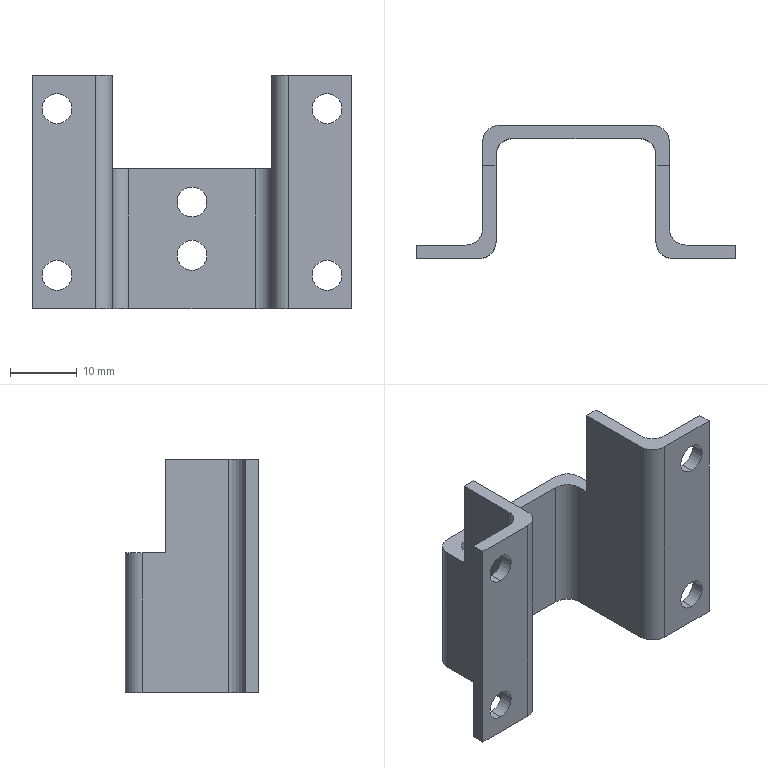Part | SolidWorks | features ICE 2, Extrusion 1 | 1 solid | 38 faces | box 48 x 20 x 35 mm | volume 4681 mm3 | cylinder 20 | plane 18 | commonest cylinder face diameters 4.5 x12 5 x8
STEP:
#1=CARTESIAN_POINT('',(0.,20.,5.75));
#2=VERTEX_POINT('',#1);
#3=CARTESIAN_POINT('',(0.,20.,10.25));
#4=VERTEX_POINT('',#3);
#5=CARTESIAN_POINT('',(0.,20.,8.));
#6=DIRECTION('',(0.,1.,0.));
#7=DIRECTION('',(0.,0.,-1.));
#8=AXIS2_PLACEMENT_3D('',#5,#6,#7);
#9=CIRCLE('',#8,2.25);
#10=EDGE_CURVE('',#2,#4,#9,.T.);
#11=ORIENTED_EDGE('',*,*,#10,.T.);
#12=CARTESIAN_POINT('',(0.,18.,10.25));
#13=VERTEX_POINT('',#12);
#14=CARTESIAN_POINT('',(0.,21.,10.25));
#15=DIRECTION('',(0.,-1.,0.));
#16=VECTOR('',#15,1000.);
#17=LINE('',#14,#16);
#18=EDGE_CURVE('',#4,#13,#17,.T.);
#19=ORIENTED_EDGE('',*,*,#18,.T.);
#20=CARTESIAN_POINT('',(0.,18.,5.75));
#21=VERTEX_POINT('',#20);
#22=CARTESIAN_POINT('',(0.,18.,8.));
#23=DIRECTION('',(0.,-1.,0.));
#24=DIRECTION('',(-1.,0.,0.));
#25=AXIS2_PLACEMENT_3D('',#22,#23,#24);
#26=CIRCLE('',#25,2.25);
#27=EDGE_CURVE('',#13,#21,#26,.T.);
#28=ORIENTED_EDGE('',*,*,#27,.T.);
#29=CARTESIAN_POINT('',(0.,21.,5.75));
#30=DIRECTION('',(0.,-1.,0.));
#31=VECTOR('',#30,1000.);
#32=LINE('',#29,#31);
#33=EDGE_CURVE('',#2,#21,#32,.T.);
#34=ORIENTED_EDGE('',*,*,#33,.F.);
#35=EDGE_LOOP('',(#11,#19,#28,#34));
#36=FACE_OUTER_BOUND('',#35,.T.);
#37=CARTESIAN_POINT('',(0.,21.,8.));
#38=DIRECTION('',(0.,-1.,0.));
#39=DIRECTION('',(0.,0.,-1.));
#40=AXIS2_PLACEMENT_3D('',#37,#38,#39);
#41=CYLINDRICAL_SURFACE('',#40,2.25);
#42=ADVANCED_FACE('',(#36),#41,.F.);
#43=CARTESIAN_POINT('',(0.,20.,13.75));
#44=VERTEX_POINT('',#43);
#45=CARTESIAN_POINT('',(0.,20.,18.25));
#46=VERTEX_POINT('',#45);
#47=CARTESIAN_POINT('',(0.,20.,16.));
#48=DIRECTION('',(0.,1.,0.));
#49=DIRECTION('',(0.,0.,-1.));
#50=AXIS2_PLACEMENT_3D('',#47,#48,#49);
#51=CIRCLE('',#50,2.25);
#52=EDGE_CURVE('',#44,#46,#51,.T.);
#53=ORIENTED_EDGE('',*,*,#52,.T.);
#54=CARTESIAN_POINT('',(0.,18.,18.25));
#55=VERTEX_POINT('',#54);
#56=CARTESIAN_POINT('',(0.,21.,18.25));
#57=DIRECTION('',(0.,-1.,0.));
#58=VECTOR('',#57,1000.);
#59=LINE('',#56,#58);
#60=EDGE_CURVE('',#46,#55,#59,.T.);
#61=ORIENTED_EDGE('',*,*,#60,.T.);
#62=CARTESIAN_POINT('',(0.,18.,13.75));
#63=VERTEX_POINT('',#62);
#64=CARTESIAN_POINT('',(0.,18.,16.));
#65=DIRECTION('',(0.,-1.,0.));
#66=DIRECTION('',(-1.,0.,0.));
#67=AXIS2_PLACEMENT_3D('',#64,#65,#66);
#68=CIRCLE('',#67,2.25);
#69=EDGE_CURVE('',#55,#63,#68,.T.);
#70=ORIENTED_EDGE('',*,*,#69,.T.);
#71=CARTESIAN_POINT('',(0.,21.,13.75));
#72=DIRECTION('',(0.,-1.,0.));
#73=VECTOR('',#72,1000.);
#74=LINE('',#71,#73);
#75=EDGE_CURVE('',#44,#63,#74,.T.);
#76=ORIENTED_EDGE('',*,*,#75,.F.);
#77=EDGE_LOOP('',(#53,#61,#70,#76));
#78=FACE_OUTER_BOUND('',#77,.T.);
#79=CARTESIAN_POINT('',(0.,21.,16.));
#80=DIRECTION('',(0.,-1.,0.));
#81=DIRECTION('',(0.,0.,-1.));
#82=AXIS2_PLACEMENT_3D('',#79,#80,#81);
#83=CYLINDRICAL_SURFACE('',#82,2.25);
#84=ADVANCED_FACE('',(#78),#83,.F.);
#85=CARTESIAN_POINT('',(20.25,2.,27.75));
#86=VERTEX_POINT('',#85);
#87=CARTESIAN_POINT('',(20.25,2.,32.25));
#88=VERTEX_POINT('',#87);
#89=CARTESIAN_POINT('',(20.25,2.,30.));
#90=DIRECTION('',(0.,1.,0.));
#91=DIRECTION('',(0.,0.,-1.));
#92=AXIS2_PLACEMENT_3D('',#89,#90,#91);
#93=CIRCLE('',#92,2.25);
#94=EDGE_CURVE('',#86,#88,#93,.T.);
#95=ORIENTED_EDGE('',*,*,#94,.T.);
#96=CARTESIAN_POINT('',(20.25,0.,32.25));
#97=VERTEX_POINT('',#96);
#98=CARTESIAN_POINT('',(20.25,21.,32.25));
#99=DIRECTION('',(0.,-1.,0.));
#100=VECTOR('',#99,1000.);
#101=LINE('',#98,#100);
#102=EDGE_CURVE('',#88,#97,#101,.T.);
#103=ORIENTED_EDGE('',*,*,#102,.T.);
#104=CARTESIAN_POINT('',(20.25,0.,27.75));
#105=VERTEX_POINT('',#104);
#106=CARTESIAN_POINT('',(20.25,0.,30.));
#107=DIRECTION('',(0.,-1.,0.));
#108=DIRECTION('',(-1.,0.,0.));
#109=AXIS2_PLACEMENT_3D('',#106,#107,#108);
#110=CIRCLE('',#109,2.25);
#111=EDGE_CURVE('',#97,#105,#110,.T.);
#112=ORIENTED_EDGE('',*,*,#111,.T.);
#113=CARTESIAN_POINT('',(20.25,21.,27.75));
#114=DIRECTION('',(0.,-1.,0.));
#115=VECTOR('',#114,1000.);
#116=LINE('',#113,#115);
#117=EDGE_CURVE('',#86,#105,#116,.T.);
#118=ORIENTED_EDGE('',*,*,#117,.F.);
#119=EDGE_LOOP('',(#95,#103,#112,#118));
#120=FACE_OUTER_BOUND('',#119,.T.);
#121=CARTESIAN_POINT('',(20.25,21.,30.));
#122=DIRECTION('',(0.,-1.,0.));
#123=DIRECTION('',(0.,0.,-1.));
#124=AXIS2_PLACEMENT_3D('',#121,#122,#123);
#125=CYLINDRICAL_SURFACE('',#124,2.25);
#126=ADVANCED_FACE('',(#120),#125,.F.);
#127=CARTESIAN_POINT('',(20.25,2.,2.75));
#128=VERTEX_POINT('',#127);
#129=CARTESIAN_POINT('',(20.25,2.,7.25));
#130=VERTEX_POINT('',#129);
#131=CARTESIAN_POINT('',(20.25,2.,5.));
#132=DIRECTION('',(0.,1.,0.));
#133=DIRECTION('',(0.,0.,-1.));
#134=AXIS2_PLACEMENT_3D('',#131,#132,#133);
#135=CIRCLE('',#134,2.25);
#136=EDGE_CURVE('',#128,#130,#135,.T.);
#137=ORIENTED_EDGE('',*,*,#136,.T.);
#138=CARTESIAN_POINT('',(20.25,0.,7.25));
#139=VERTEX_POINT('',#138);
#140=CARTESIAN_POINT('',(20.25,21.,7.25));
#141=DIRECTION('',(0.,-1.,0.));
#142=VECTOR('',#141,1000.);
#143=LINE('',#140,#142);
#144=EDGE_CURVE('',#130,#139,#143,.T.);
#145=ORIENTED_EDGE('',*,*,#144,.T.);
#146=CARTESIAN_POINT('',(20.25,0.,2.75));
#147=VERTEX_POINT('',#146);
#148=CARTESIAN_POINT('',(20.25,0.,5.));
#149=DIRECTION('',(0.,-1.,0.));
#150=DIRECTION('',(-1.,0.,0.));
#151=AXIS2_PLACEMENT_3D('',#148,#149,#150);
#152=CIRCLE('',#151,2.25);
#153=EDGE_CURVE('',#139,#147,#152,.T.);
#154=ORIENTED_EDGE('',*,*,#153,.T.);
#155=CARTESIAN_POINT('',(20.25,21.,2.75));
#156=DIRECTION('',(0.,-1.,0.));
#157=VECTOR('',#156,1000.);
#158=LINE('',#155,#157);
#159=EDGE_CURVE('',#128,#147,#158,.T.);
#160=ORIENTED_EDGE('',*,*,#159,.F.);
#161=EDGE_LOOP('',(#137,#145,#154,#160));
#162=FACE_OUTER_BOUND('',#161,.T.);
#163=CARTESIAN_POINT('',(20.25,21.,5.));
#164=DIRECTION('',(0.,-1.,0.));
#165=DIRECTION('',(0.,0.,-1.));
#166=AXIS2_PLACEMENT_3D('',#163,#164,#165);
#167=CYLINDRICAL_SURFACE('',#166,2.25);
#168=ADVANCED_FACE('',(#162),#167,.F.);
#169=CARTESIAN_POINT('',(-20.25,2.,27.75));
#170=VERTEX_POINT('',#169);
#171=CARTESIAN_POINT('',(-20.25,2.,32.25));
#172=VERTEX_POINT('',#171);
#173=CARTESIAN_POINT('',(-20.25,2.,30.));
#174=DIRECTION('',(0.,1.,0.));
#175=DIRECTION('',(0.,0.,-1.));
#176=AXIS2_PLACEMENT_3D('',#173,#174,#175);
#177=CIRCLE('',#176,2.25);
#178=EDGE_CURVE('',#170,#172,#177,.T.);
#179=ORIENTED_EDGE('',*,*,#178,.T.);
#180=CARTESIAN_POINT('',(-20.25,0.,32.25));
#181=VERTEX_POINT('',#180);
#182=CARTESIAN_POINT('',(-20.25,21.,32.25));
#183=DIRECTION('',(0.,-1.,0.));
#184=VECTOR('',#183,1000.);
#185=LINE('',#182,#184);
#186=EDGE_CURVE('',#172,#181,#185,.T.);
#187=ORIENTED_EDGE('',*,*,#186,.T.);
#188=CARTESIAN_POINT('',(-20.25,0.,27.75));
#189=VERTEX_POINT('',#188);
#190=CARTESIAN_POINT('',(-20.25,0.,30.));
#191=DIRECTION('',(0.,-1.,0.));
#192=DIRECTION('',(0.,0.,1.));
#193=AXIS2_PLACEMENT_3D('',#190,#191,#192);
#194=CIRCLE('',#193,2.25);
#195=EDGE_CURVE('',#181,#189,#194,.T.);
#196=ORIENTED_EDGE('',*,*,#195,.T.);
#197=CARTESIAN_POINT('',(-20.25,21.,27.75));
#198=DIRECTION('',(0.,-1.,0.));
#199=VECTOR('',#198,1000.);
#200=LINE('',#197,#199);
#201=EDGE_CURVE('',#170,#189,#200,.T.);
#202=ORIENTED_EDGE('',*,*,#201,.F.);
#203=EDGE_LOOP('',(#179,#187,#196,#202));
#204=FACE_OUTER_BOUND('',#203,.T.);
#205=CARTESIAN_POINT('',(-20.25,21.,30.));
#206=DIRECTION('',(0.,-1.,0.));
#207=DIRECTION('',(0.,0.,-1.));
#208=AXIS2_PLACEMENT_3D('',#205,#206,#207);
#209=CYLINDRICAL_SURFACE('',#208,2.25);
#210=ADVANCED_FACE('',(#204),#209,.F.);
#211=CARTESIAN_POINT('',(-20.25,2.,2.75));
#212=VERTEX_POINT('',#211);
#213=CARTESIAN_POINT('',(-20.25,2.,7.25));
#214=VERTEX_POINT('',#213);
#215=CARTESIAN_POINT('',(-20.25,2.,5.));
#216=DIRECTION('',(0.,1.,0.));
#217=DIRECTION('',(0.,0.,-1.));
#218=AXIS2_PLACEMENT_3D('',#215,#216,#217);
#219=CIRCLE('',#218,2.25);
#220=EDGE_CURVE('',#212,#214,#219,.T.);
#221=ORIENTED_EDGE('',*,*,#220,.T.);
#222=CARTESIAN_POINT('',(-20.25,0.,7.25));
#223=VERTEX_POINT('',#222);
#224=CARTESIAN_POINT('',(-20.25,21.,7.25));
#225=DIRECTION('',(0.,-1.,0.));
#226=VECTOR('',#225,1000.);
#227=LINE('',#224,#226);
#228=EDGE_CURVE('',#214,#223,#227,.T.);
#229=ORIENTED_EDGE('',*,*,#228,.T.);
#230=CARTESIAN_POINT('',(-20.25,0.,2.75));
#231=VERTEX_POINT('',#230);
#232=CARTESIAN_POINT('',(-20.25,0.,5.));
#233=DIRECTION('',(0.,-1.,0.));
#234=DIRECTION('',(0.,0.,1.));
#235=AXIS2_PLACEMENT_3D('',#232,#233,#234);
#236=CIRCLE('',#235,2.25);
#237=EDGE_CURVE('',#223,#231,#236,.T.);
#238=ORIENTED_EDGE('',*,*,#237,.T.);
#239=CARTESIAN_POINT('',(-20.25,21.,2.75));
#240=DIRECTION('',(0.,-1.,0.));
#241=VECTOR('',#240,1000.);
#242=LINE('',#239,#241);
#243=EDGE_CURVE('',#212,#231,#242,.T.);
#244=ORIENTED_EDGE('',*,*,#243,.F.);
#245=EDGE_LOOP('',(#221,#229,#238,#244));
#246=FACE_OUTER_BOUND('',#245,.T.);
#247=CARTESIAN_POINT('',(-20.25,21.,5.));
#248=DIRECTION('',(0.,-1.,0.));
#249=DIRECTION('',(0.,0.,-1.));
#250=AXIS2_PLACEMENT_3D('',#247,#248,#249);
#251=CYLINDRICAL_SURFACE('',#250,2.25);
#252=ADVANCED_FACE('',(#246),#251,.F.);
#253=CARTESIAN_POINT('',(-12.,15.5,21.));
#254=VERTEX_POINT('',#253);
#255=CARTESIAN_POINT('',(-9.5,18.,21.));
#256=VERTEX_POINT('',#255);
#257=CARTESIAN_POINT('',(-9.5,15.5,21.));
#258=DIRECTION('',(0.,0.,-1.));
#259=DIRECTION('',(1.,0.,0.));
#260=AXIS2_PLACEMENT_3D('',#257,#258,#259);
#261=CIRCLE('',#260,2.5);
#262=EDGE_CURVE('',#254,#256,#261,.T.);
#263=ORIENTED_EDGE('',*,*,#262,.F.);
#264=CARTESIAN_POINT('',(-12.,15.5,0.));
#265=VERTEX_POINT('',#264);
#266=CARTESIAN_POINT('',(-12.,15.5,35.));
#267=DIRECTION('',(0.,0.,-1.));
#268=VECTOR('',#267,1000.);
#269=LINE('',#266,#268);
#270=EDGE_CURVE('',#254,#265,#269,.T.);
#271=ORIENTED_EDGE('',*,*,#270,.T.);
#272=CARTESIAN_POINT('',(-9.5,18.,0.));
#273=VERTEX_POINT('',#272);
#274=CARTESIAN_POINT('',(-9.5,15.5,0.));
#275=DIRECTION('',(0.,0.,-1.));
#276=DIRECTION('',(-1.,0.,0.));
#277=AXIS2_PLACEMENT_3D('',#274,#275,#276);
#278=CIRCLE('',#277,2.5);
#279=EDGE_CURVE('',#265,#273,#278,.T.);
#280=ORIENTED_EDGE('',*,*,#279,.T.);
#281=CARTESIAN_POINT('',(-9.5,18.,35.));
#282=DIRECTION('',(0.,0.,-1.));
#283=VECTOR('',#282,1000.);
#284=LINE('',#281,#283);
#285=EDGE_CURVE('',#256,#273,#284,.T.);
#286=ORIENTED_EDGE('',*,*,#285,.F.);
#287=EDGE_LOOP('',(#263,#271,#280,#286));
#288=FACE_OUTER_BOUND('',#287,.T.);
#289=CARTESIAN_POINT('',(-9.5,15.5,35.));
#290=DIRECTION('',(0.,0.,-1.));
#291=DIRECTION('',(-1.,0.,0.));
#292=AXIS2_PLACEMENT_3D('',#289,#290,#291);
#293=CYLINDRICAL_SURFACE('',#292,2.5);
#294=ADVANCED_FACE('',(#288),#293,.F.);
#295=CARTESIAN_POINT('',(0.,18.,8.));
#296=DIRECTION('',(0.,-1.,0.));
#297=DIRECTION('',(-1.,0.,0.));
#298=AXIS2_PLACEMENT_3D('',#295,#296,#297);
#299=CIRCLE('',#298,2.25);
#300=EDGE_CURVE('',#21,#13,#299,.T.);
#301=ORIENTED_EDGE('',*,*,#300,.F.);
#302=ORIENTED_EDGE('',*,*,#27,.F.);
#303=EDGE_LOOP('',(#301,#302));
#304=FACE_BOUND('',#303,.T.);
#305=CARTESIAN_POINT('',(0.,18.,16.));
#306=DIRECTION('',(0.,-1.,0.));
#307=DIRECTION('',(-1.,0.,0.));
#308=AXIS2_PLACEMENT_3D('',#305,#306,#307);
#309=CIRCLE('',#308,2.25);
#310=EDGE_CURVE('',#63,#55,#309,.T.);
#311=ORIENTED_EDGE('',*,*,#310,.F.);
#312=ORIENTED_EDGE('',*,*,#69,.F.);
#313=EDGE_LOOP('',(#311,#312));
#314=FACE_BOUND('',#313,.T.);
#315=CARTESIAN_POINT('',(9.5,18.,21.));
#316=VERTEX_POINT('',#315);
#317=CARTESIAN_POINT('',(-9.5,18.,21.));
#318=DIRECTION('',(1.,0.,0.));
#319=VECTOR('',#318,1000.);
#320=LINE('',#317,#319);
#321=EDGE_CURVE('',#256,#316,#320,.T.);
#322=ORIENTED_EDGE('',*,*,#321,.F.);
#323=ORIENTED_EDGE('',*,*,#285,.T.);
#324=CARTESIAN_POINT('',(9.5,18.,0.));
#325=VERTEX_POINT('',#324);
#326=CARTESIAN_POINT('',(-9.5,18.,0.));
#327=DIRECTION('',(1.,0.,0.));
#328=VECTOR('',#327,1000.);
#329=LINE('',#326,#328);
#330=EDGE_CURVE('',#273,#325,#329,.T.);
#331=ORIENTED_EDGE('',*,*,#330,.T.);
#332=CARTESIAN_POINT('',(9.5,18.,35.));
#333=DIRECTION('',(0.,0.,-1.));
#334=VECTOR('',#333,1000.);
#335=LINE('',#332,#334);
#336=EDGE_CURVE('',#316,#325,#335,.T.);
#337=ORIENTED_EDGE('',*,*,#336,.F.);
#338=EDGE_LOOP('',(#322,#323,#331,#337));
#339=FACE_OUTER_BOUND('',#338,.T.);
#340=CARTESIAN_POINT('',(-9.5,18.,35.));
#341=DIRECTION('',(0.,1.,0.));
#342=DIRECTION('',(-1.,0.,0.));
#343=AXIS2_PLACEMENT_3D('',#340,#341,#342);
#344=PLANE('',#343);
#345=ADVANCED_FACE('',(#304,#314,#339),#344,.F.);
#346=CARTESIAN_POINT('',(12.,15.5,21.));
#347=VERTEX_POINT('',#346);
#348=CARTESIAN_POINT('',(9.5,15.5,21.));
#349=DIRECTION('',(0.,0.,-1.));
#350=DIRECTION('',(1.,0.,0.));
#351=AXIS2_PLACEMENT_3D('',#348,#349,#350);
#352=CIRCLE('',#351,2.5);
#353=EDGE_CURVE('',#316,#347,#352,.T.);
#354=ORIENTED_EDGE('',*,*,#353,.F.);
#355=ORIENTED_EDGE('',*,*,#336,.T.);
#356=CARTESIAN_POINT('',(12.,15.5,0.));
#357=VERTEX_POINT('',#356);
#358=CARTESIAN_POINT('',(9.5,15.5,0.));
#359=DIRECTION('',(0.,0.,-1.));
#360=DIRECTION('',(1.,0.,0.));
#361=AXIS2_PLACEMENT_3D('',#358,#359,#360);
#362=CIRCLE('',#361,2.5);
#363=EDGE_CURVE('',#325,#357,#362,.T.);
#364=ORIENTED_EDGE('',*,*,#363,.T.);
#365=CARTESIAN_POINT('',(12.,15.5,35.));
#366=DIRECTION('',(0.,0.,-1.));
#367=VECTOR('',#366,1000.);
#368=LINE('',#365,#367);
#369=EDGE_CURVE('',#347,#357,#368,.T.);
#370=ORIENTED_EDGE('',*,*,#369,.F.);
#371=EDGE_LOOP('',(#354,#355,#364,#370));
#372=FACE_OUTER_BOUND('',#371,.T.);
#373=CARTESIAN_POINT('',(9.5,15.5,35.));
#374=DIRECTION('',(0.,0.,-1.));
#375=DIRECTION('',(-1.,0.,0.));
#376=AXIS2_PLACEMENT_3D('',#373,#374,#375);
#377=CYLINDRICAL_SURFACE('',#376,2.5);
#378=ADVANCED_FACE('',(#372),#377,.F.);
#379=CARTESIAN_POINT('',(14.,17.5,21.));
#380=VERTEX_POINT('',#379);
#381=CARTESIAN_POINT('',(11.5,20.,21.));
#382=VERTEX_POINT('',#381);
#383=CARTESIAN_POINT('',(11.5,17.5,21.));
#384=DIRECTION('',(0.,0.,1.));
#385=DIRECTION('',(1.,0.,0.));
#386=AXIS2_PLACEMENT_3D('',#383,#384,#385);
#387=CIRCLE('',#386,2.5);
#388=EDGE_CURVE('',#380,#382,#387,.T.);
#389=ORIENTED_EDGE('',*,*,#388,.F.);
#390=CARTESIAN_POINT('',(14.,17.5,0.));
#391=VERTEX_POINT('',#390);
#392=CARTESIAN_POINT('',(14.,17.5,35.));
#393=DIRECTION('',(0.,0.,-1.));
#394=VECTOR('',#393,1000.);
#395=LINE('',#392,#394);
#396=EDGE_CURVE('',#380,#391,#395,.T.);
#397=ORIENTED_EDGE('',*,*,#396,.T.);
#398=CARTESIAN_POINT('',(11.5,20.,0.));
#399=VERTEX_POINT('',#398);
#400=CARTESIAN_POINT('',(11.5,17.5,0.));
#401=DIRECTION('',(0.,0.,1.));
#402=DIRECTION('',(1.,0.,0.));
#403=AXIS2_PLACEMENT_3D('',#400,#401,#402);
#404=CIRCLE('',#403,2.5);
#405=EDGE_CURVE('',#391,#399,#404,.T.);
#406=ORIENTED_EDGE('',*,*,#405,.T.);
#407=CARTESIAN_POINT('',(11.5,20.,35.));
#408=DIRECTION('',(0.,0.,-1.));
#409=VECTOR('',#408,1000.);
#410=LINE('',#407,#409);
#411=EDGE_CURVE('',#382,#399,#410,.T.);
#412=ORIENTED_EDGE('',*,*,#411,.F.);
#413=EDGE_LOOP('',(#389,#397,#406,#412));
#414=FACE_OUTER_BOUND('',#413,.T.);
#415=CARTESIAN_POINT('',(11.5,17.5,35.));
#416=DIRECTION('',(0.,0.,-1.));
#417=DIRECTION('',(-1.,0.,0.));
#418=AXIS2_PLACEMENT_3D('',#415,#416,#417);
#419=CYLINDRICAL_SURFACE('',#418,2.5);
#420=ADVANCED_FACE('',(#414),#419,.T.);
#421=ORIENTED_EDGE('',*,*,#10,.F.);
#422=CARTESIAN_POINT('',(0.,20.,8.));
#423=DIRECTION('',(0.,1.,0.));
#424=DIRECTION('',(0.,0.,-1.));
#425=AXIS2_PLACEMENT_3D('',#422,#423,#424);
#426=CIRCLE('',#425,2.25);
#427=EDGE_CURVE('',#4,#2,#426,.T.);
#428=ORIENTED_EDGE('',*,*,#427,.F.);
#429=EDGE_LOOP('',(#421,#428));
#430=FACE_BOUND('',#429,.T.);
#431=ORIENTED_EDGE('',*,*,#52,.F.);
#432=CARTESIAN_POINT('',(0.,20.,16.));
#433=DIRECTION('',(0.,1.,0.));
#434=DIRECTION('',(0.,0.,-1.));
#435=AXIS2_PLACEMENT_3D('',#432,#433,#434);
#436=CIRCLE('',#435,2.25);
#437=EDGE_CURVE('',#46,#44,#436,.T.);
#438=ORIENTED_EDGE('',*,*,#437,.F.);
#439=EDGE_LOOP('',(#431,#438));
#440=FACE_BOUND('',#439,.T.);
#441=CARTESIAN_POINT('',(-11.5,20.,21.));
#442=VERTEX_POINT('',#441);
#443=CARTESIAN_POINT('',(-11.5,20.,21.));
#444=DIRECTION('',(-1.,0.,0.));
#445=VECTOR('',#444,1000.);
#446=LINE('',#443,#445);
#447=EDGE_CURVE('',#382,#442,#446,.T.);
#448=ORIENTED_EDGE('',*,*,#447,.F.);
#449=ORIENTED_EDGE('',*,*,#411,.T.);
#450=CARTESIAN_POINT('',(-11.5,20.,0.));
#451=VERTEX_POINT('',#450);
#452=CARTESIAN_POINT('',(-11.5,20.,0.));
#453=DIRECTION('',(-1.,0.,0.));
#454=VECTOR('',#453,1000.);
#455=LINE('',#452,#454);
#456=EDGE_CURVE('',#399,#451,#455,.T.);
#457=ORIENTED_EDGE('',*,*,#456,.T.);
#458=CARTESIAN_POINT('',(-11.5,20.,35.));
#459=DIRECTION('',(0.,0.,-1.));
#460=VECTOR('',#459,1000.);
#461=LINE('',#458,#460);
#462=EDGE_CURVE('',#442,#451,#461,.T.);
#463=ORIENTED_EDGE('',*,*,#462,.F.);
#464=EDGE_LOOP('',(#448,#449,#457,#463));
#465=FACE_OUTER_BOUND('',#464,.T.);
#466=CARTESIAN_POINT('',(-11.5,20.,35.));
#467=DIRECTION('',(0.,-1.,0.));
#468=DIRECTION('',(0.,0.,-1.));
#469=AXIS2_PLACEMENT_3D('',#466,#467,#468);
#470=PLANE('',#469);
#471=ADVANCED_FACE('',(#430,#440,#465),#470,.F.);
#472=CARTESIAN_POINT('',(-14.,17.5,21.));
#473=VERTEX_POINT('',#472);
#474=CARTESIAN_POINT('',(-11.5,17.5,21.));
#475=DIRECTION('',(0.,0.,1.));
#476=DIRECTION('',(1.,0.,0.));
#477=AXIS2_PLACEMENT_3D('',#474,#475,#476);
#478=CIRCLE('',#477,2.5);
#479=EDGE_CURVE('',#442,#473,#478,.T.);
#480=ORIENTED_EDGE('',*,*,#479,.F.);
#481=ORIENTED_EDGE('',*,*,#462,.T.);
#482=CARTESIAN_POINT('',(-14.,17.5,0.));
#483=VERTEX_POINT('',#482);
#484=CARTESIAN_POINT('',(-11.5,17.5,0.));
#485=DIRECTION('',(0.,0.,1.));
#486=DIRECTION('',(-1.,0.,0.));
#487=AXIS2_PLACEMENT_3D('',#484,#485,#486);
#488=CIRCLE('',#487,2.5);
#489=EDGE_CURVE('',#451,#483,#488,.T.);
#490=ORIENTED_EDGE('',*,*,#489,.T.);
#491=CARTESIAN_POINT('',(-14.,17.5,35.));
#492=DIRECTION('',(0.,0.,-1.));
#493=VECTOR('',#492,1000.);
#494=LINE('',#491,#493);
#495=EDGE_CURVE('',#473,#483,#494,.T.);
#496=ORIENTED_EDGE('',*,*,#495,.F.);
#497=EDGE_LOOP('',(#480,#481,#490,#496));
#498=FACE_OUTER_BOUND('',#497,.T.);
#499=CARTESIAN_POINT('',(-11.5,17.5,35.));
#500=DIRECTION('',(0.,0.,-1.));
#501=DIRECTION('',(-1.,0.,0.));
#502=AXIS2_PLACEMENT_3D('',#499,#500,#501);
#503=CYLINDRICAL_SURFACE('',#502,2.5);
#504=ADVANCED_FACE('',(#498),#503,.T.);
#505=CARTESIAN_POINT('',(-14.,14.,35.));
#506=VERTEX_POINT('',#505);
#507=CARTESIAN_POINT('',(-12.,14.,35.));
#508=VERTEX_POINT('',#507);
#509=CARTESIAN_POINT('',(-14.5,14.,35.));
#510=DIRECTION('',(1.,0.,0.));
#511=VECTOR('',#510,1000.);
#512=LINE('',#509,#511);
#513=EDGE_CURVE('',#506,#508,#512,.T.);
#514=ORIENTED_EDGE('',*,*,#513,.F.);
#515=CARTESIAN_POINT('',(-14.,4.5,35.));
#516=VERTEX_POINT('',#515);
#517=CARTESIAN_POINT('',(-14.,4.5,35.));
#518=DIRECTION('',(0.,-1.,0.));
#519=VECTOR('',#518,1000.);
#520=LINE('',#517,#519);
#521=EDGE_CURVE('',#506,#516,#520,.T.);
#522=ORIENTED_EDGE('',*,*,#521,.T.);
#523=CARTESIAN_POINT('',(-16.5,2.,35.));
#524=VERTEX_POINT('',#523);
#525=CARTESIAN_POINT('',(-16.5,4.5,35.));
#526=DIRECTION('',(0.,0.,-1.));
#527=DIRECTION('',(1.,0.,0.));
#528=AXIS2_PLACEMENT_3D('',#525,#526,#527);
#529=CIRCLE('',#528,2.5);
#530=EDGE_CURVE('',#516,#524,#529,.T.);
#531=ORIENTED_EDGE('',*,*,#530,.T.);
#532=CARTESIAN_POINT('',(-24.,2.,35.));
#533=VERTEX_POINT('',#532);
#534=CARTESIAN_POINT('',(-24.,2.,35.));
#535=DIRECTION('',(-1.,0.,0.));
#536=VECTOR('',#535,1000.);
#537=LINE('',#534,#536);
#538=EDGE_CURVE('',#524,#533,#537,.T.);
#539=ORIENTED_EDGE('',*,*,#538,.T.);
#540=CARTESIAN_POINT('',(-24.,0.,35.));
#541=VERTEX_POINT('',#540);
#542=CARTESIAN_POINT('',(-24.,2.,35.));
#543=DIRECTION('',(0.,-1.,0.));
#544=VECTOR('',#543,1000.);
#545=LINE('',#542,#544);
#546=EDGE_CURVE('',#533,#541,#545,.T.);
#547=ORIENTED_EDGE('',*,*,#546,.T.);
#548=CARTESIAN_POINT('',(-14.5,0.,35.));
#549=VERTEX_POINT('',#548);
#550=CARTESIAN_POINT('',(-24.,0.,35.));
#551=DIRECTION('',(1.,0.,0.));
#552=VECTOR('',#551,1000.);
#553=LINE('',#550,#552);
#554=EDGE_CURVE('',#541,#549,#553,.T.);
#555=ORIENTED_EDGE('',*,*,#554,.T.);
#556=CARTESIAN_POINT('',(-12.,2.5,35.));
#557=VERTEX_POINT('',#556);
#558=CARTESIAN_POINT('',(-14.5,2.5,35.));
#559=DIRECTION('',(0.,0.,1.));
#560=DIRECTION('',(1.,0.,0.));
#561=AXIS2_PLACEMENT_3D('',#558,#559,#560);
#562=CIRCLE('',#561,2.5);
#563=EDGE_CURVE('',#549,#557,#562,.T.);
#564=ORIENTED_EDGE('',*,*,#563,.T.);
#565=CARTESIAN_POINT('',(-12.,2.5,35.));
#566=DIRECTION('',(0.,1.,0.));
#567=VECTOR('',#566,1000.);
#568=LINE('',#565,#567);
#569=EDGE_CURVE('',#557,#508,#568,.T.);
#570=ORIENTED_EDGE('',*,*,#569,.T.);
#571=EDGE_LOOP('',(#514,#522,#531,#539,#547,#555,#564,#570));
#572=FACE_OUTER_BOUND('',#571,.T.);
#573=CARTESIAN_POINT('',(-14.5,2.5,35.));
#574=DIRECTION('',(0.,0.,1.));
#575=DIRECTION('',(1.,0.,0.));
#576=AXIS2_PLACEMENT_3D('',#573,#574,#575);
#577=PLANE('',#576);
#578=ADVANCED_FACE('',(#572),#577,.T.);
#579=CARTESIAN_POINT('',(-24.,2.,0.));
#580=VERTEX_POINT('',#579);
#581=CARTESIAN_POINT('',(-24.,0.,0.));
#582=VERTEX_POINT('',#581);
#583=CARTESIAN_POINT('',(-24.,2.,0.));
#584=DIRECTION('',(0.,-1.,0.));
#585=VECTOR('',#584,1000.);
#586=LINE('',#583,#585);
#587=EDGE_CURVE('',#580,#582,#586,.T.);
#588=ORIENTED_EDGE('',*,*,#587,.T.);
#589=CARTESIAN_POINT('',(-24.,0.,35.));
#590=DIRECTION('',(0.,0.,-1.));
#591=VECTOR('',#590,1000.);
#592=LINE('',#589,#591);
#593=EDGE_CURVE('',#541,#582,#592,.T.);
#594=ORIENTED_EDGE('',*,*,#593,.F.);
#595=ORIENTED_EDGE('',*,*,#546,.F.);
#596=CARTESIAN_POINT('',(-24.,2.,35.));
#597=DIRECTION('',(0.,0.,-1.));
#598=VECTOR('',#597,1000.);
#599=LINE('',#596,#598);
#600=EDGE_CURVE('',#533,#580,#599,.T.);
#601=ORIENTED_EDGE('',*,*,#600,.T.);
#602=EDGE_LOOP('',(#588,#594,#595,#601));
#603=FACE_OUTER_BOUND('',#602,.T.);
#604=CARTESIAN_POINT('',(-24.,2.,35.));
#605=DIRECTION('',(1.,0.,0.));
#606=DIRECTION('',(0.,0.,-1.));
#607=AXIS2_PLACEMENT_3D('',#604,#605,#606);
#608=PLANE('',#607);
#609=ADVANCED_FACE('',(#603),#608,.F.);
#610=CARTESIAN_POINT('',(-20.25,0.,30.));
#611=DIRECTION('',(0.,-1.,0.));
#612=DIRECTION('',(0.,0.,1.));
#613=AXIS2_PLACEMENT_3D('',#610,#611,#612);
#614=CIRCLE('',#613,2.25);
#615=EDGE_CURVE('',#189,#181,#614,.T.);
#616=ORIENTED_EDGE('',*,*,#615,.F.);
#617=ORIENTED_EDGE('',*,*,#195,.F.);
#618=EDGE_LOOP('',(#616,#617));
#619=FACE_BOUND('',#618,.T.);
#620=CARTESIAN_POINT('',(-20.25,0.,5.));
#621=DIRECTION('',(0.,-1.,0.));
#622=DIRECTION('',(0.,0.,1.));
#623=AXIS2_PLACEMENT_3D('',#620,#621,#622);
#624=CIRCLE('',#623,2.25);
#625=EDGE_CURVE('',#231,#223,#624,.T.);
#626=ORIENTED_EDGE('',*,*,#625,.F.);
#627=ORIENTED_EDGE('',*,*,#237,.F.);
#628=EDGE_LOOP('',(#626,#627));
#629=FACE_BOUND('',#628,.T.);
#630=CARTESIAN_POINT('',(-14.5,0.,0.));
#631=VERTEX_POINT('',#630);
#632=CARTESIAN_POINT('',(-24.,0.,0.));
#633=DIRECTION('',(1.,0.,0.));
#634=VECTOR('',#633,1000.);
#635=LINE('',#632,#634);
#636=EDGE_CURVE('',#582,#631,#635,.T.);
#637=ORIENTED_EDGE('',*,*,#636,.T.);
#638=CARTESIAN_POINT('',(-14.5,0.,35.));
#639=DIRECTION('',(0.,0.,-1.));
#640=VECTOR('',#639,1000.);
#641=LINE('',#638,#640);
#642=EDGE_CURVE('',#549,#631,#641,.T.);
#643=ORIENTED_EDGE('',*,*,#642,.F.);
#644=ORIENTED_EDGE('',*,*,#554,.F.);
#645=ORIENTED_EDGE('',*,*,#593,.T.);
#646=EDGE_LOOP('',(#637,#643,#644,#645));
#647=FACE_OUTER_BOUND('',#646,.T.);
#648=CARTESIAN_POINT('',(-24.,0.,35.));
#649=DIRECTION('',(0.,1.,0.));
#650=DIRECTION('',(0.,0.,1.));
#651=AXIS2_PLACEMENT_3D('',#648,#649,#650);
#652=PLANE('',#651);
#653=ADVANCED_FACE('',(#619,#629,#647),#652,.F.);
#654=CARTESIAN_POINT('',(-12.,2.5,0.));
#655=VERTEX_POINT('',#654);
#656=CARTESIAN_POINT('',(-14.5,2.5,0.));
#657=DIRECTION('',(0.,0.,1.));
#658=DIRECTION('',(1.,0.,0.));
#659=AXIS2_PLACEMENT_3D('',#656,#657,#658);
#660=CIRCLE('',#659,2.5);
#661=EDGE_CURVE('',#631,#655,#660,.T.);
#662=ORIENTED_EDGE('',*,*,#661,.T.);
#663=CARTESIAN_POINT('',(-12.,2.5,35.));
#664=DIRECTION('',(0.,0.,-1.));
#665=VECTOR('',#664,1000.);
#666=LINE('',#663,#665);
#667=EDGE_CURVE('',#557,#655,#666,.T.);
#668=ORIENTED_EDGE('',*,*,#667,.F.);
#669=ORIENTED_EDGE('',*,*,#563,.F.);
#670=ORIENTED_EDGE('',*,*,#642,.T.);
#671=EDGE_LOOP('',(#662,#668,#669,#670));
#672=FACE_OUTER_BOUND('',#671,.T.);
#673=CARTESIAN_POINT('',(-14.5,2.5,35.));
#674=DIRECTION('',(0.,0.,-1.));
#675=DIRECTION('',(-1.,0.,0.));
#676=AXIS2_PLACEMENT_3D('',#673,#674,#675);
#677=CYLINDRICAL_SURFACE('',#676,2.5);
#678=ADVANCED_FACE('',(#672),#677,.T.);
#679=CARTESIAN_POINT('',(-12.,14.,21.));
#680=VERTEX_POINT('',#679);
#681=CARTESIAN_POINT('',(-12.,2.5,21.));
#682=DIRECTION('',(0.,1.,0.));
#683=VECTOR('',#682,1000.);
#684=LINE('',#681,#683);
#685=EDGE_CURVE('',#680,#254,#684,.T.);
#686=ORIENTED_EDGE('',*,*,#685,.F.);
#687=CARTESIAN_POINT('',(-12.,14.,35.));
#688=DIRECTION('',(0.,0.,1.));
#689=VECTOR('',#688,1000.);
#690=LINE('',#687,#689);
#691=EDGE_CURVE('',#680,#508,#690,.T.);
#692=ORIENTED_EDGE('',*,*,#691,.T.);
#693=ORIENTED_EDGE('',*,*,#569,.F.);
#694=ORIENTED_EDGE('',*,*,#667,.T.);
#695=CARTESIAN_POINT('',(-12.,2.5,0.));
#696=DIRECTION('',(0.,1.,0.));
#697=VECTOR('',#696,1000.);
#698=LINE('',#695,#697);
#699=EDGE_CURVE('',#655,#265,#698,.T.);
#700=ORIENTED_EDGE('',*,*,#699,.T.);
#701=ORIENTED_EDGE('',*,*,#270,.F.);
#702=EDGE_LOOP('',(#686,#692,#693,#694,#700,#701));
#703=FACE_OUTER_BOUND('',#702,.T.);
#704=CARTESIAN_POINT('',(-12.,2.5,35.));
#705=DIRECTION('',(-1.,0.,0.));
#706=DIRECTION('',(0.,0.,1.));
#707=AXIS2_PLACEMENT_3D('',#704,#705,#706);
#708=PLANE('',#707);
#709=ADVANCED_FACE('',(#703),#708,.F.);
#710=CARTESIAN_POINT('',(12.,14.,35.));
#711=VERTEX_POINT('',#710);
#712=CARTESIAN_POINT('',(12.,2.5,35.));
#713=VERTEX_POINT('',#712);
#714=CARTESIAN_POINT('',(12.,15.5,35.));
#715=DIRECTION('',(0.,-1.,0.));
#716=VECTOR('',#715,1000.);
#717=LINE('',#714,#716);
#718=EDGE_CURVE('',#711,#713,#717,.T.);
#719=ORIENTED_EDGE('',*,*,#718,.F.);
#720=CARTESIAN_POINT('',(12.,14.,21.));
#721=VERTEX_POINT('',#720);
#722=CARTESIAN_POINT('',(12.,14.,35.));
#723=DIRECTION('',(0.,0.,-1.));
#724=VECTOR('',#723,1000.);
#725=LINE('',#722,#724);
#726=EDGE_CURVE('',#711,#721,#725,.T.);
#727=ORIENTED_EDGE('',*,*,#726,.T.);
#728=CARTESIAN_POINT('',(12.,15.5,21.));
#729=DIRECTION('',(0.,-1.,0.));
#730=VECTOR('',#729,1000.);
#731=LINE('',#728,#730);
#732=EDGE_CURVE('',#347,#721,#731,.T.);
#733=ORIENTED_EDGE('',*,*,#732,.F.);
#734=ORIENTED_EDGE('',*,*,#369,.T.);
#735=CARTESIAN_POINT('',(12.,2.5,0.));
#736=VERTEX_POINT('',#735);
#737=CARTESIAN_POINT('',(12.,15.5,0.));
#738=DIRECTION('',(0.,-1.,0.));
#739=VECTOR('',#738,1000.);
#740=LINE('',#737,#739);
#741=EDGE_CURVE('',#357,#736,#740,.T.);
#742=ORIENTED_EDGE('',*,*,#741,.T.);
#743=CARTESIAN_POINT('',(12.,2.5,35.));
#744=DIRECTION('',(0.,0.,-1.));
#745=VECTOR('',#744,1000.);
#746=LINE('',#743,#745);
#747=EDGE_CURVE('',#713,#736,#746,.T.);
#748=ORIENTED_EDGE('',*,*,#747,.F.);
#749=EDGE_LOOP('',(#719,#727,#733,#734,#742,#748));
#750=FACE_OUTER_BOUND('',#749,.T.);
#751=CARTESIAN_POINT('',(12.,15.5,35.));
#752=DIRECTION('',(1.,0.,0.));
#753=DIRECTION('',(0.,1.,0.));
#754=AXIS2_PLACEMENT_3D('',#751,#752,#753);
#755=PLANE('',#754);
#756=ADVANCED_FACE('',(#750),#755,.F.);
#757=CARTESIAN_POINT('',(14.5,0.,0.));
#758=VERTEX_POINT('',#757);
#759=CARTESIAN_POINT('',(14.5,2.5,0.));
#760=DIRECTION('',(0.,0.,1.));
#761=DIRECTION('',(1.,0.,0.));
#762=AXIS2_PLACEMENT_3D('',#759,#760,#761);
#763=CIRCLE('',#762,2.5);
#764=EDGE_CURVE('',#736,#758,#763,.T.);
#765=ORIENTED_EDGE('',*,*,#764,.T.);
#766=CARTESIAN_POINT('',(14.5,0.,35.));
#767=VERTEX_POINT('',#766);
#768=CARTESIAN_POINT('',(14.5,0.,35.));
#769=DIRECTION('',(0.,0.,-1.));
#770=VECTOR('',#769,1000.);
#771=LINE('',#768,#770);
#772=EDGE_CURVE('',#767,#758,#771,.T.);
#773=ORIENTED_EDGE('',*,*,#772,.F.);
#774=CARTESIAN_POINT('',(14.5,2.5,35.));
#775=DIRECTION('',(0.,0.,1.));
#776=DIRECTION('',(1.,0.,0.));
#777=AXIS2_PLACEMENT_3D('',#774,#775,#776);
#778=CIRCLE('',#777,2.5);
#779=EDGE_CURVE('',#713,#767,#778,.T.);
#780=ORIENTED_EDGE('',*,*,#779,.F.);
#781=ORIENTED_EDGE('',*,*,#747,.T.);
#782=EDGE_LOOP('',(#765,#773,#780,#781));
#783=FACE_OUTER_BOUND('',#782,.T.);
#784=CARTESIAN_POINT('',(14.5,2.5,35.));
#785=DIRECTION('',(0.,0.,-1.));
#786=DIRECTION('',(-1.,0.,0.));
#787=AXIS2_PLACEMENT_3D('',#784,#785,#786);
#788=CYLINDRICAL_SURFACE('',#787,2.5);
#789=ADVANCED_FACE('',(#783),#788,.T.);
#790=CARTESIAN_POINT('',(20.25,0.,30.));
#791=DIRECTION('',(0.,-1.,0.));
#792=DIRECTION('',(-1.,0.,0.));
#793=AXIS2_PLACEMENT_3D('',#790,#791,#792);
#794=CIRCLE('',#793,2.25);
#795=EDGE_CURVE('',#105,#97,#794,.T.);
#796=ORIENTED_EDGE('',*,*,#795,.F.);
#797=ORIENTED_EDGE('',*,*,#111,.F.);
#798=EDGE_LOOP('',(#796,#797));
#799=FACE_BOUND('',#798,.T.);
#800=CARTESIAN_POINT('',(20.25,0.,5.));
#801=DIRECTION('',(0.,-1.,0.));
#802=DIRECTION('',(-1.,0.,0.));
#803=AXIS2_PLACEMENT_3D('',#800,#801,#802);
#804=CIRCLE('',#803,2.25);
#805=EDGE_CURVE('',#147,#139,#804,.T.);
#806=ORIENTED_EDGE('',*,*,#805,.F.);
#807=ORIENTED_EDGE('',*,*,#153,.F.);
#808=EDGE_LOOP('',(#806,#807));
#809=FACE_BOUND('',#808,.T.);
#810=CARTESIAN_POINT('',(24.,0.,0.));
#811=VERTEX_POINT('',#810);
#812=CARTESIAN_POINT('',(14.5,0.,0.));
#813=DIRECTION('',(1.,0.,0.));
#814=VECTOR('',#813,1000.);
#815=LINE('',#812,#814);
#816=EDGE_CURVE('',#758,#811,#815,.T.);
#817=ORIENTED_EDGE('',*,*,#816,.T.);
#818=CARTESIAN_POINT('',(24.,0.,35.));
#819=VERTEX_POINT('',#818);
#820=CARTESIAN_POINT('',(24.,0.,35.));
#821=DIRECTION('',(0.,0.,-1.));
#822=VECTOR('',#821,1000.);
#823=LINE('',#820,#822);
#824=EDGE_CURVE('',#819,#811,#823,.T.);
#825=ORIENTED_EDGE('',*,*,#824,.F.);
#826=CARTESIAN_POINT('',(14.5,0.,35.));
#827=DIRECTION('',(1.,0.,0.));
#828=VECTOR('',#827,1000.);
#829=LINE('',#826,#828);
#830=EDGE_CURVE('',#767,#819,#829,.T.);
#831=ORIENTED_EDGE('',*,*,#830,.F.);
#832=ORIENTED_EDGE('',*,*,#772,.T.);
#833=EDGE_LOOP('',(#817,#825,#831,#832));
#834=FACE_OUTER_BOUND('',#833,.T.);
#835=CARTESIAN_POINT('',(14.5,0.,35.));
#836=DIRECTION('',(0.,1.,0.));
#837=DIRECTION('',(-1.,0.,0.));
#838=AXIS2_PLACEMENT_3D('',#835,#836,#837);
#839=PLANE('',#838);
#840=ADVANCED_FACE('',(#799,#809,#834),#839,.F.);
#841=CARTESIAN_POINT('',(24.,2.,0.));
#842=VERTEX_POINT('',#841);
#843=CARTESIAN_POINT('',(24.,2.,0.));
#844=DIRECTION('',(0.,1.,0.));
#845=VECTOR('',#844,1000.);
#846=LINE('',#843,#845);
#847=EDGE_CURVE('',#811,#842,#846,.T.);
#848=ORIENTED_EDGE('',*,*,#847,.T.);
#849=CARTESIAN_POINT('',(24.,2.,35.));
#850=VERTEX_POINT('',#849);
#851=CARTESIAN_POINT('',(24.,2.,35.));
#852=DIRECTION('',(0.,0.,-1.));
#853=VECTOR('',#852,1000.);
#854=LINE('',#851,#853);
#855=EDGE_CURVE('',#850,#842,#854,.T.);
#856=ORIENTED_EDGE('',*,*,#855,.F.);
#857=CARTESIAN_POINT('',(24.,2.,35.));
#858=DIRECTION('',(0.,1.,0.));
#859=VECTOR('',#858,1000.);
#860=LINE('',#857,#859);
#861=EDGE_CURVE('',#819,#850,#860,.T.);
#862=ORIENTED_EDGE('',*,*,#861,.F.);
#863=ORIENTED_EDGE('',*,*,#824,.T.);
#864=EDGE_LOOP('',(#848,#856,#862,#863));
#865=FACE_OUTER_BOUND('',#864,.T.);
#866=CARTESIAN_POINT('',(24.,2.,35.));
#867=DIRECTION('',(-1.,0.,0.));
#868=DIRECTION('',(0.,0.,1.));
#869=AXIS2_PLACEMENT_3D('',#866,#867,#868);
#870=PLANE('',#869);
#871=ADVANCED_FACE('',(#865),#870,.F.);
#872=ORIENTED_EDGE('',*,*,#94,.F.);
#873=CARTESIAN_POINT('',(20.25,2.,30.));
#874=DIRECTION('',(0.,1.,0.));
#875=DIRECTION('',(0.,0.,-1.));
#876=AXIS2_PLACEMENT_3D('',#873,#874,#875);
#877=CIRCLE('',#876,2.25);
#878=EDGE_CURVE('',#88,#86,#877,.T.);
#879=ORIENTED_EDGE('',*,*,#878,.F.);
#880=EDGE_LOOP('',(#872,#879));
#881=FACE_BOUND('',#880,.T.);
#882=ORIENTED_EDGE('',*,*,#136,.F.);
#883=CARTESIAN_POINT('',(20.25,2.,5.));
#884=DIRECTION('',(0.,1.,0.));
#885=DIRECTION('',(0.,0.,-1.));
#886=AXIS2_PLACEMENT_3D('',#883,#884,#885);
#887=CIRCLE('',#886,2.25);
#888=EDGE_CURVE('',#130,#128,#887,.T.);
#889=ORIENTED_EDGE('',*,*,#888,.F.);
#890=EDGE_LOOP('',(#882,#889));
#891=FACE_BOUND('',#890,.T.);
#892=CARTESIAN_POINT('',(16.5,2.,0.));
#893=VERTEX_POINT('',#892);
#894=CARTESIAN_POINT('',(16.5,2.,0.));
#895=DIRECTION('',(-1.,0.,0.));
#896=VECTOR('',#895,1000.);
#897=LINE('',#894,#896);
#898=EDGE_CURVE('',#842,#893,#897,.T.);
#899=ORIENTED_EDGE('',*,*,#898,.T.);
#900=CARTESIAN_POINT('',(16.5,2.,35.));
#901=VERTEX_POINT('',#900);
#902=CARTESIAN_POINT('',(16.5,2.,35.));
#903=DIRECTION('',(0.,0.,-1.));
#904=VECTOR('',#903,1000.);
#905=LINE('',#902,#904);
#906=EDGE_CURVE('',#901,#893,#905,.T.);
#907=ORIENTED_EDGE('',*,*,#906,.F.);
#908=CARTESIAN_POINT('',(16.5,2.,35.));
#909=DIRECTION('',(-1.,0.,0.));
#910=VECTOR('',#909,1000.);
#911=LINE('',#908,#910);
#912=EDGE_CURVE('',#850,#901,#911,.T.);
#913=ORIENTED_EDGE('',*,*,#912,.F.);
#914=ORIENTED_EDGE('',*,*,#855,.T.);
#915=EDGE_LOOP('',(#899,#907,#913,#914));
#916=FACE_OUTER_BOUND('',#915,.T.);
#917=CARTESIAN_POINT('',(16.5,2.,35.));
#918=DIRECTION('',(0.,-1.,0.));
#919=DIRECTION('',(0.,0.,-1.));
#920=AXIS2_PLACEMENT_3D('',#917,#918,#919);
#921=PLANE('',#920);
#922=ADVANCED_FACE('',(#881,#891,#916),#921,.F.);
#923=CARTESIAN_POINT('',(14.,4.5,0.));
#924=VERTEX_POINT('',#923);
#925=CARTESIAN_POINT('',(16.5,4.5,0.));
#926=DIRECTION('',(0.,0.,-1.));
#927=DIRECTION('',(-1.,0.,0.));
#928=AXIS2_PLACEMENT_3D('',#925,#926,#927);
#929=CIRCLE('',#928,2.5);
#930=EDGE_CURVE('',#893,#924,#929,.T.);
#931=ORIENTED_EDGE('',*,*,#930,.T.);
#932=CARTESIAN_POINT('',(14.,4.5,35.));
#933=VERTEX_POINT('',#932);
#934=CARTESIAN_POINT('',(14.,4.5,35.));
#935=DIRECTION('',(0.,0.,-1.));
#936=VECTOR('',#935,1000.);
#937=LINE('',#934,#936);
#938=EDGE_CURVE('',#933,#924,#937,.T.);
#939=ORIENTED_EDGE('',*,*,#938,.F.);
#940=CARTESIAN_POINT('',(16.5,4.5,35.));
#941=DIRECTION('',(0.,0.,-1.));
#942=DIRECTION('',(-1.,0.,0.));
#943=AXIS2_PLACEMENT_3D('',#940,#941,#942);
#944=CIRCLE('',#943,2.5);
#945=EDGE_CURVE('',#901,#933,#944,.T.);
#946=ORIENTED_EDGE('',*,*,#945,.F.);
#947=ORIENTED_EDGE('',*,*,#906,.T.);
#948=EDGE_LOOP('',(#931,#939,#946,#947));
#949=FACE_OUTER_BOUND('',#948,.T.);
#950=CARTESIAN_POINT('',(16.5,4.5,35.));
#951=DIRECTION('',(0.,0.,-1.));
#952=DIRECTION('',(-1.,0.,0.));
#953=AXIS2_PLACEMENT_3D('',#950,#951,#952);
#954=CYLINDRICAL_SURFACE('',#953,2.5);
#955=ADVANCED_FACE('',(#949),#954,.F.);
#956=CARTESIAN_POINT('',(14.,14.,21.));
#957=VERTEX_POINT('',#956);
#958=CARTESIAN_POINT('',(14.,17.5,21.));
#959=DIRECTION('',(0.,1.,0.));
#960=VECTOR('',#959,1000.);
#961=LINE('',#958,#960);
#962=EDGE_CURVE('',#957,#380,#961,.T.);
#963=ORIENTED_EDGE('',*,*,#962,.F.);
#964=CARTESIAN_POINT('',(14.,14.,35.));
#965=VERTEX_POINT('',#964);
#966=CARTESIAN_POINT('',(14.,14.,35.));
#967=DIRECTION('',(0.,0.,1.));
#968=VECTOR('',#967,1000.);
#969=LINE('',#966,#968);
#970=EDGE_CURVE('',#957,#965,#969,.T.);
#971=ORIENTED_EDGE('',*,*,#970,.T.);
#972=CARTESIAN_POINT('',(14.,17.5,35.));
#973=DIRECTION('',(0.,1.,0.));
#974=VECTOR('',#973,1000.);
#975=LINE('',#972,#974);
#976=EDGE_CURVE('',#933,#965,#975,.T.);
#977=ORIENTED_EDGE('',*,*,#976,.F.);
#978=ORIENTED_EDGE('',*,*,#938,.T.);
#979=CARTESIAN_POINT('',(14.,17.5,0.));
#980=DIRECTION('',(0.,1.,0.));
#981=VECTOR('',#980,1000.);
#982=LINE('',#979,#981);
#983=EDGE_CURVE('',#924,#391,#982,.T.);
#984=ORIENTED_EDGE('',*,*,#983,.T.);
#985=ORIENTED_EDGE('',*,*,#396,.F.);
#986=EDGE_LOOP('',(#963,#971,#977,#978,#984,#985));
#987=FACE_OUTER_BOUND('',#986,.T.);
#988=CARTESIAN_POINT('',(14.,17.5,35.));
#989=DIRECTION('',(-1.,0.,0.));
#990=DIRECTION('',(0.,-1.,0.));
#991=AXIS2_PLACEMENT_3D('',#988,#989,#990);
#992=PLANE('',#991);
#993=ADVANCED_FACE('',(#987),#992,.F.);
#994=ORIENTED_EDGE('',*,*,#521,.F.);
#995=CARTESIAN_POINT('',(-14.,14.,21.));
#996=VERTEX_POINT('',#995);
#997=CARTESIAN_POINT('',(-14.,14.,35.));
#998=DIRECTION('',(0.,0.,-1.));
#999=VECTOR('',#998,1000.);
#1000=LINE('',#997,#999);
#1001=EDGE_CURVE('',#506,#996,#1000,.T.);
#1002=ORIENTED_EDGE('',*,*,#1001,.T.);
#1003=CARTESIAN_POINT('',(-14.,4.5,21.));
#1004=DIRECTION('',(0.,-1.,0.));
#1005=VECTOR('',#1004,1000.);
#1006=LINE('',#1003,#1005);
#1007=EDGE_CURVE('',#473,#996,#1006,.T.);
#1008=ORIENTED_EDGE('',*,*,#1007,.F.);
#1009=ORIENTED_EDGE('',*,*,#495,.T.);
#1010=CARTESIAN_POINT('',(-14.,4.5,0.));
#1011=VERTEX_POINT('',#1010);
#1012=CARTESIAN_POINT('',(-14.,4.5,0.));
#1013=DIRECTION('',(0.,-1.,0.));
#1014=VECTOR('',#1013,1000.);
#1015=LINE('',#1012,#1014);
#1016=EDGE_CURVE('',#483,#1011,#1015,.T.);
#1017=ORIENTED_EDGE('',*,*,#1016,.T.);
#1018=CARTESIAN_POINT('',(-14.,4.5,35.));
#1019=DIRECTION('',(0.,0.,-1.));
#1020=VECTOR('',#1019,1000.);
#1021=LINE('',#1018,#1020);
#1022=EDGE_CURVE('',#516,#1011,#1021,.T.);
#1023=ORIENTED_EDGE('',*,*,#1022,.F.);
#1024=EDGE_LOOP('',(#994,#1002,#1008,#1009,#1017,#1023));
#1025=FACE_OUTER_BOUND('',#1024,.T.);
#1026=CARTESIAN_POINT('',(-14.,4.5,35.));
#1027=DIRECTION('',(1.,0.,0.));
#1028=DIRECTION('',(0.,0.,-1.));
#1029=AXIS2_PLACEMENT_3D('',#1026,#1027,#1028);
#1030=PLANE('',#1029);
#1031=ADVANCED_FACE('',(#1025),#1030,.F.);
#1032=CARTESIAN_POINT('',(-16.5,2.,0.));
#1033=VERTEX_POINT('',#1032);
#1034=CARTESIAN_POINT('',(-16.5,4.5,0.));
#1035=DIRECTION('',(0.,0.,-1.));
#1036=DIRECTION('',(1.,0.,0.));
#1037=AXIS2_PLACEMENT_3D('',#1034,#1035,#1036);
#1038=CIRCLE('',#1037,2.5);
#1039=EDGE_CURVE('',#1011,#1033,#1038,.T.);
#1040=ORIENTED_EDGE('',*,*,#1039,.T.);
#1041=CARTESIAN_POINT('',(-16.5,2.,35.));
#1042=DIRECTION('',(0.,0.,-1.));
#1043=VECTOR('',#1042,1000.);
#1044=LINE('',#1041,#1043);
#1045=EDGE_CURVE('',#524,#1033,#1044,.T.);
#1046=ORIENTED_EDGE('',*,*,#1045,.F.);
#1047=ORIENTED_EDGE('',*,*,#530,.F.);
#1048=ORIENTED_EDGE('',*,*,#1022,.T.);
#1049=EDGE_LOOP('',(#1040,#1046,#1047,#1048));
#1050=FACE_OUTER_BOUND('',#1049,.T.);
#1051=CARTESIAN_POINT('',(-16.5,4.5,35.));
#1052=DIRECTION('',(0.,0.,-1.));
#1053=DIRECTION('',(-1.,0.,0.));
#1054=AXIS2_PLACEMENT_3D('',#1051,#1052,#1053);
#1055=CYLINDRICAL_SURFACE('',#1054,2.5);
#1056=ADVANCED_FACE('',(#1050),#1055,.F.);
#1057=ORIENTED_EDGE('',*,*,#178,.F.);
#1058=CARTESIAN_POINT('',(-20.25,2.,30.));
#1059=DIRECTION('',(0.,1.,0.));
#1060=DIRECTION('',(0.,0.,-1.));
#1061=AXIS2_PLACEMENT_3D('',#1058,#1059,#1060);
#1062=CIRCLE('',#1061,2.25);
#1063=EDGE_CURVE('',#172,#170,#1062,.T.);
#1064=ORIENTED_EDGE('',*,*,#1063,.F.);
#1065=EDGE_LOOP('',(#1057,#1064));
#1066=FACE_BOUND('',#1065,.T.);
#1067=ORIENTED_EDGE('',*,*,#220,.F.);
#1068=CARTESIAN_POINT('',(-20.25,2.,5.));
#1069=DIRECTION('',(0.,1.,0.));
#1070=DIRECTION('',(0.,0.,-1.));
#1071=AXIS2_PLACEMENT_3D('',#1068,#1069,#1070);
#1072=CIRCLE('',#1071,2.25);
#1073=EDGE_CURVE('',#214,#212,#1072,.T.);
#1074=ORIENTED_EDGE('',*,*,#1073,.F.);
#1075=EDGE_LOOP('',(#1067,#1074));
#1076=FACE_BOUND('',#1075,.T.);
#1077=CARTESIAN_POINT('',(-24.,2.,0.));
#1078=DIRECTION('',(-1.,0.,0.));
#1079=VECTOR('',#1078,1000.);
#1080=LINE('',#1077,#1079);
#1081=EDGE_CURVE('',#1033,#580,#1080,.T.);
#1082=ORIENTED_EDGE('',*,*,#1081,.T.);
#1083=ORIENTED_EDGE('',*,*,#600,.F.);
#1084=ORIENTED_EDGE('',*,*,#538,.F.);
#1085=ORIENTED_EDGE('',*,*,#1045,.T.);
#1086=EDGE_LOOP('',(#1082,#1083,#1084,#1085));
#1087=FACE_OUTER_BOUND('',#1086,.T.);
#1088=CARTESIAN_POINT('',(-24.,2.,35.));
#1089=DIRECTION('',(0.,-1.,0.));
#1090=DIRECTION('',(0.,0.,-1.));
#1091=AXIS2_PLACEMENT_3D('',#1088,#1089,#1090);
#1092=PLANE('',#1091);
#1093=ADVANCED_FACE('',(#1066,#1076,#1087),#1092,.F.);
#1094=CARTESIAN_POINT('',(-14.5,14.,35.));
#1095=DIRECTION('',(1.,0.,0.));
#1096=VECTOR('',#1095,1000.);
#1097=LINE('',#1094,#1096);
#1098=EDGE_CURVE('',#711,#965,#1097,.T.);
#1099=ORIENTED_EDGE('',*,*,#1098,.F.);
#1100=ORIENTED_EDGE('',*,*,#718,.T.);
#1101=ORIENTED_EDGE('',*,*,#779,.T.);
#1102=ORIENTED_EDGE('',*,*,#830,.T.);
#1103=ORIENTED_EDGE('',*,*,#861,.T.);
#1104=ORIENTED_EDGE('',*,*,#912,.T.);
#1105=ORIENTED_EDGE('',*,*,#945,.T.);
#1106=ORIENTED_EDGE('',*,*,#976,.T.);
#1107=EDGE_LOOP('',(#1099,#1100,#1101,#1102,#1103,#1104,#1105,#1106));
#1108=FACE_OUTER_BOUND('',#1107,.T.);
#1109=CARTESIAN_POINT('',(-14.5,2.5,35.));
#1110=DIRECTION('',(0.,0.,1.));
#1111=DIRECTION('',(1.,0.,0.));
#1112=AXIS2_PLACEMENT_3D('',#1109,#1110,#1111);
#1113=PLANE('',#1112);
#1114=ADVANCED_FACE('',(#1108),#1113,.T.);
#1115=ORIENTED_EDGE('',*,*,#587,.F.);
#1116=ORIENTED_EDGE('',*,*,#1081,.F.);
#1117=ORIENTED_EDGE('',*,*,#1039,.F.);
#1118=ORIENTED_EDGE('',*,*,#1016,.F.);
#1119=ORIENTED_EDGE('',*,*,#489,.F.);
#1120=ORIENTED_EDGE('',*,*,#456,.F.);
#1121=ORIENTED_EDGE('',*,*,#405,.F.);
#1122=ORIENTED_EDGE('',*,*,#983,.F.);
#1123=ORIENTED_EDGE('',*,*,#930,.F.);
#1124=ORIENTED_EDGE('',*,*,#898,.F.);
#1125=ORIENTED_EDGE('',*,*,#847,.F.);
#1126=ORIENTED_EDGE('',*,*,#816,.F.);
#1127=ORIENTED_EDGE('',*,*,#764,.F.);
#1128=ORIENTED_EDGE('',*,*,#741,.F.);
#1129=ORIENTED_EDGE('',*,*,#363,.F.);
#1130=ORIENTED_EDGE('',*,*,#330,.F.);
#1131=ORIENTED_EDGE('',*,*,#279,.F.);
#1132=ORIENTED_EDGE('',*,*,#699,.F.);
#1133=ORIENTED_EDGE('',*,*,#661,.F.);
#1134=ORIENTED_EDGE('',*,*,#636,.F.);
#1135=EDGE_LOOP('',(#1115,#1116,#1117,#1118,#1119,#1120,#1121,#1122,#1123,#1124,#1125,#1126,#1127,#1128,#1129,#1130,#1131,#1132,#1133,#1134));
#1136=FACE_OUTER_BOUND('',#1135,.T.);
#1137=CARTESIAN_POINT('',(-14.5,2.5,0.));
#1138=DIRECTION('',(0.,0.,1.));
#1139=DIRECTION('',(1.,0.,0.));
#1140=AXIS2_PLACEMENT_3D('',#1137,#1138,#1139);
#1141=PLANE('',#1140);
#1142=ADVANCED_FACE('',(#1136),#1141,.F.);
#1143=ORIENTED_EDGE('',*,*,#685,.T.);
#1144=ORIENTED_EDGE('',*,*,#262,.T.);
#1145=ORIENTED_EDGE('',*,*,#321,.T.);
#1146=ORIENTED_EDGE('',*,*,#353,.T.);
#1147=ORIENTED_EDGE('',*,*,#732,.T.);
#1148=CARTESIAN_POINT('',(17.196,14.,21.));
#1149=DIRECTION('',(1.,0.,0.));
#1150=VECTOR('',#1149,1000.);
#1151=LINE('',#1148,#1150);
#1152=EDGE_CURVE('',#721,#957,#1151,.T.);
#1153=ORIENTED_EDGE('',*,*,#1152,.T.);
#1154=ORIENTED_EDGE('',*,*,#962,.T.);
#1155=ORIENTED_EDGE('',*,*,#388,.T.);
#1156=ORIENTED_EDGE('',*,*,#447,.T.);
#1157=ORIENTED_EDGE('',*,*,#479,.T.);
#1158=ORIENTED_EDGE('',*,*,#1007,.T.);
#1159=CARTESIAN_POINT('',(17.196,14.,21.));
#1160=DIRECTION('',(1.,0.,0.));
#1161=VECTOR('',#1160,1000.);
#1162=LINE('',#1159,#1161);
#1163=EDGE_CURVE('',#996,#680,#1162,.T.);
#1164=ORIENTED_EDGE('',*,*,#1163,.T.);
#1165=EDGE_LOOP('',(#1143,#1144,#1145,#1146,#1147,#1153,#1154,#1155,#1156,#1157,#1158,#1164));
#1166=FACE_OUTER_BOUND('',#1165,.T.);
#1167=CARTESIAN_POINT('',(0.,0.,21.));
#1168=DIRECTION('',(0.,0.,1.));
#1169=DIRECTION('',(1.,0.,0.));
#1170=AXIS2_PLACEMENT_3D('',#1167,#1168,#1169);
#1171=PLANE('',#1170);
#1172=ADVANCED_FACE('',(#1166),#1171,.T.);
#1173=ORIENTED_EDGE('',*,*,#1163,.F.);
#1174=ORIENTED_EDGE('',*,*,#1001,.F.);
#1175=ORIENTED_EDGE('',*,*,#513,.T.);
#1176=ORIENTED_EDGE('',*,*,#691,.F.);
#1177=EDGE_LOOP('',(#1173,#1174,#1175,#1176));
#1178=FACE_OUTER_BOUND('',#1177,.T.);
#1179=CARTESIAN_POINT('',(17.196,14.,21.));
#1180=DIRECTION('',(0.,-1.,0.));
#1181=DIRECTION('',(1.,0.,0.));
#1182=AXIS2_PLACEMENT_3D('',#1179,#1180,#1181);
#1183=PLANE('',#1182);
#1184=ADVANCED_FACE('',(#1178),#1183,.F.);
#1185=ORIENTED_EDGE('',*,*,#1098,.T.);
#1186=ORIENTED_EDGE('',*,*,#970,.F.);
#1187=ORIENTED_EDGE('',*,*,#1152,.F.);
#1188=ORIENTED_EDGE('',*,*,#726,.F.);
#1189=EDGE_LOOP('',(#1185,#1186,#1187,#1188));
#1190=FACE_OUTER_BOUND('',#1189,.T.);
#1191=CARTESIAN_POINT('',(17.196,14.,21.));
#1192=DIRECTION('',(0.,-1.,0.));
#1193=DIRECTION('',(1.,0.,0.));
#1194=AXIS2_PLACEMENT_3D('',#1191,#1192,#1193);
#1195=PLANE('',#1194);
#1196=ADVANCED_FACE('',(#1190),#1195,.F.);
#1197=ORIENTED_EDGE('',*,*,#228,.F.);
#1198=ORIENTED_EDGE('',*,*,#1073,.T.);
#1199=ORIENTED_EDGE('',*,*,#243,.T.);
#1200=ORIENTED_EDGE('',*,*,#625,.T.);
#1201=EDGE_LOOP('',(#1197,#1198,#1199,#1200));
#1202=FACE_OUTER_BOUND('',#1201,.T.);
#1203=CARTESIAN_POINT('',(-20.25,21.,5.));
#1204=DIRECTION('',(0.,-1.,0.));
#1205=DIRECTION('',(0.,0.,-1.));
#1206=AXIS2_PLACEMENT_3D('',#1203,#1204,#1205);
#1207=CYLINDRICAL_SURFACE('',#1206,2.25);
#1208=ADVANCED_FACE('',(#1202),#1207,.F.);
#1209=ORIENTED_EDGE('',*,*,#186,.F.);
#1210=ORIENTED_EDGE('',*,*,#1063,.T.);
#1211=ORIENTED_EDGE('',*,*,#201,.T.);
#1212=ORIENTED_EDGE('',*,*,#615,.T.);
#1213=EDGE_LOOP('',(#1209,#1210,#1211,#1212));
#1214=FACE_OUTER_BOUND('',#1213,.T.);
#1215=CARTESIAN_POINT('',(-20.25,21.,30.));
#1216=DIRECTION('',(0.,-1.,0.));
#1217=DIRECTION('',(0.,0.,-1.));
#1218=AXIS2_PLACEMENT_3D('',#1215,#1216,#1217);
#1219=CYLINDRICAL_SURFACE('',#1218,2.25);
#1220=ADVANCED_FACE('',(#1214),#1219,.F.);
#1221=ORIENTED_EDGE('',*,*,#144,.F.);
#1222=ORIENTED_EDGE('',*,*,#888,.T.);
#1223=ORIENTED_EDGE('',*,*,#159,.T.);
#1224=ORIENTED_EDGE('',*,*,#805,.T.);
#1225=EDGE_LOOP('',(#1221,#1222,#1223,#1224));
#1226=FACE_OUTER_BOUND('',#1225,.T.);
#1227=CARTESIAN_POINT('',(20.25,21.,5.));
#1228=DIRECTION('',(0.,-1.,0.));
#1229=DIRECTION('',(0.,0.,-1.));
#1230=AXIS2_PLACEMENT_3D('',#1227,#1228,#1229);
#1231=CYLINDRICAL_SURFACE('',#1230,2.25);
#1232=ADVANCED_FACE('',(#1226),#1231,.F.);
#1233=ORIENTED_EDGE('',*,*,#102,.F.);
#1234=ORIENTED_EDGE('',*,*,#878,.T.);
#1235=ORIENTED_EDGE('',*,*,#117,.T.);
#1236=ORIENTED_EDGE('',*,*,#795,.T.);
#1237=EDGE_LOOP('',(#1233,#1234,#1235,#1236));
#1238=FACE_OUTER_BOUND('',#1237,.T.);
#1239=CARTESIAN_POINT('',(20.25,21.,30.));
#1240=DIRECTION('',(0.,-1.,0.));
#1241=DIRECTION('',(0.,0.,-1.));
#1242=AXIS2_PLACEMENT_3D('',#1239,#1240,#1241);
#1243=CYLINDRICAL_SURFACE('',#1242,2.25);
#1244=ADVANCED_FACE('',(#1238),#1243,.F.);
#1245=ORIENTED_EDGE('',*,*,#60,.F.);
#1246=ORIENTED_EDGE('',*,*,#437,.T.);
#1247=ORIENTED_EDGE('',*,*,#75,.T.);
#1248=ORIENTED_EDGE('',*,*,#310,.T.);
#1249=EDGE_LOOP('',(#1245,#1246,#1247,#1248));
#1250=FACE_OUTER_BOUND('',#1249,.T.);
#1251=CARTESIAN_POINT('',(0.,21.,16.));
#1252=DIRECTION('',(0.,-1.,0.));
#1253=DIRECTION('',(0.,0.,-1.));
#1254=AXIS2_PLACEMENT_3D('',#1251,#1252,#1253);
#1255=CYLINDRICAL_SURFACE('',#1254,2.25);
#1256=ADVANCED_FACE('',(#1250),#1255,.F.);
#1257=ORIENTED_EDGE('',*,*,#18,.F.);
#1258=ORIENTED_EDGE('',*,*,#427,.T.);
#1259=ORIENTED_EDGE('',*,*,#33,.T.);
#1260=ORIENTED_EDGE('',*,*,#300,.T.);
#1261=EDGE_LOOP('',(#1257,#1258,#1259,#1260));
#1262=FACE_OUTER_BOUND('',#1261,.T.);
#1263=CARTESIAN_POINT('',(0.,21.,8.));
#1264=DIRECTION('',(0.,-1.,0.));
#1265=DIRECTION('',(0.,0.,-1.));
#1266=AXIS2_PLACEMENT_3D('',#1263,#1264,#1265);
#1267=CYLINDRICAL_SURFACE('',#1266,2.25);
#1268=ADVANCED_FACE('',(#1262),#1267,.F.);
#1269=CLOSED_SHELL('',(#42,#84,#126,#168,#210,#252,#294,#345,#378,#420,#471,#504,#578,#609,#653,#678,#709,#756,#789,#840,#871,#922,#955,#993,#1031,#1056,#1093,#1114,#1142,#1172,#1184,#1196,#1208,#1220,#1232,#1244,#1256,#1268));
#1270=MANIFOLD_SOLID_BREP('',#1269);
#1271=CARTESIAN_POINT('',(0.,0.,0.));
#1272=DIRECTION('',(0.,0.,1.));
#1273=DIRECTION('',(1.,0.,0.));
#1274=AXIS2_PLACEMENT_3D('',#1271,#1272,#1273);
#1275=(LENGTH_UNIT()NAMED_UNIT(*)SI_UNIT(.MILLI.,.METRE.));
#1276=UNCERTAINTY_MEASURE_WITH_UNIT(LENGTH_MEASURE(0.00001),#1275,'','');
#1277=(NAMED_UNIT(*)PLANE_ANGLE_UNIT()SI_UNIT($,.RADIAN.));
#1278=(NAMED_UNIT(*)SI_UNIT($,.STERADIAN.)SOLID_ANGLE_UNIT());
#1279=(GEOMETRIC_REPRESENTATION_CONTEXT(3)GLOBAL_UNCERTAINTY_ASSIGNED_CONTEXT((#1276))GLOBAL_UNIT_ASSIGNED_CONTEXT((#1275,#1277,#1278))REPRESENTATION_CONTEXT('',''));
#1280=ADVANCED_BREP_SHAPE_REPRESENTATION('',(#1270,#1274),#1279);